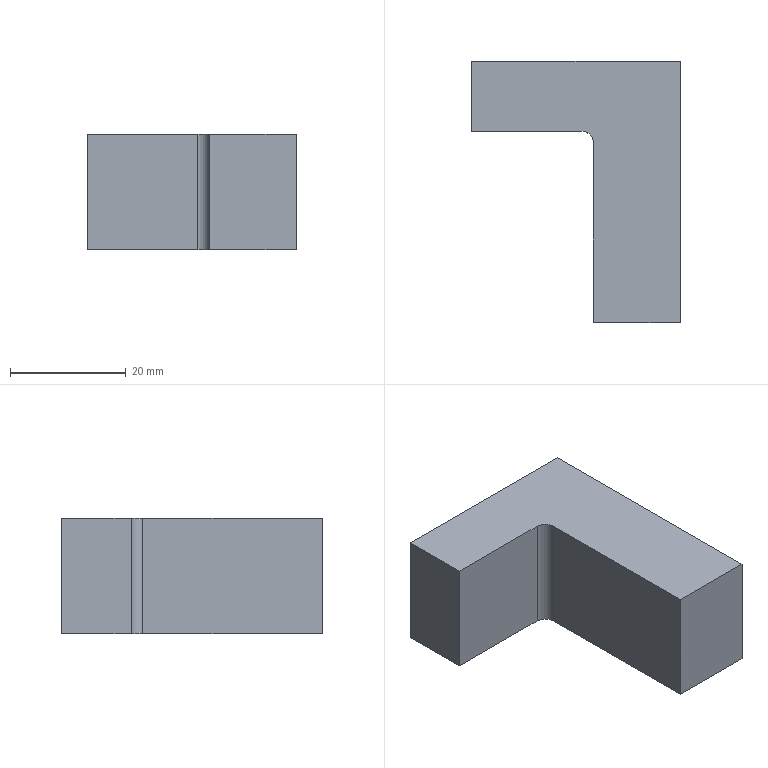Part | STEP file | 001-003-Shaft storage cylinder connection block | 1 solid | 9 faces | box 36 x 45 x 20 mm | volume 18557 mm3 | plane 8 | cylinder 1 | commonest cylinder face diameters 4 x1
STEP:
#1=CARTESIAN_POINT('',(0.,0.,0.));
#2=DIRECTION('',(0.,0.,1.));
#3=DIRECTION('',(1.,0.,0.));
#4=AXIS2_PLACEMENT_3D('',#1,#2,#3);
#5=CARTESIAN_POINT('',(18.,-22.5,0.));
#6=VERTEX_POINT('',#5);
#7=CARTESIAN_POINT('',(18.,22.5,0.));
#8=VERTEX_POINT('',#7);
#9=CARTESIAN_POINT('',(18.,-22.5,0.));
#10=DIRECTION('',(0.,1.,0.));
#11=VECTOR('',#10,1.);
#12=LINE('',#9,#11);
#13=CARTESIAN_POINT('',(18.,-22.5,20.));
#14=DIRECTION('',(-1.,0.,0.));
#15=DIRECTION('',(0.,0.,1.));
#16=AXIS2_PLACEMENT_3D('',#13,#14,#15);
#17=PLANE('',#16);
#18=CARTESIAN_POINT('',(-20.,0.));
#19=DIRECTION('',(0.,1.));
#20=VECTOR('',#19,1.);
#21=LINE('',#18,#20);
#22=(GEOMETRIC_REPRESENTATION_CONTEXT(2)PARAMETRIC_REPRESENTATION_CONTEXT()REPRESENTATION_CONTEXT('',''));
#23=DEFINITIONAL_REPRESENTATION('',(#21),#22);
#24=PCURVE('',#17,#23);
#25=CARTESIAN_POINT('',(0.,0.,0.));
#26=DIRECTION('',(0.,0.,-1.));
#27=DIRECTION('',(-1.,0.,0.));
#28=AXIS2_PLACEMENT_3D('',#25,#26,#27);
#29=PLANE('',#28);
#30=CARTESIAN_POINT('',(-18.,-22.5));
#31=DIRECTION('',(0.,1.));
#32=VECTOR('',#31,1.);
#33=LINE('',#30,#32);
#34=(GEOMETRIC_REPRESENTATION_CONTEXT(2)PARAMETRIC_REPRESENTATION_CONTEXT()REPRESENTATION_CONTEXT('',''));
#35=DEFINITIONAL_REPRESENTATION('',(#33),#34);
#36=PCURVE('',#29,#35);
#37=SURFACE_CURVE('',#12,(#24,#36),.PCURVE_S1.);
#38=EDGE_CURVE('',#6,#8,#37,.T.);
#39=ORIENTED_EDGE('',*,*,#38,.T.);
#40=CARTESIAN_POINT('',(18.,22.5,20.));
#41=VERTEX_POINT('',#40);
#42=CARTESIAN_POINT('',(18.,22.5,20.));
#43=DIRECTION('',(0.,0.,-1.));
#44=VECTOR('',#43,1.);
#45=LINE('',#42,#44);
#46=CARTESIAN_POINT('',(0.,45.));
#47=DIRECTION('',(-1.,0.));
#48=VECTOR('',#47,1.);
#49=LINE('',#46,#48);
#50=(GEOMETRIC_REPRESENTATION_CONTEXT(2)PARAMETRIC_REPRESENTATION_CONTEXT()REPRESENTATION_CONTEXT('',''));
#51=DEFINITIONAL_REPRESENTATION('',(#49),#50);
#52=PCURVE('',#17,#51);
#53=CARTESIAN_POINT('',(-18.,22.5,20.));
#54=DIRECTION('',(0.,-1.,0.));
#55=DIRECTION('',(0.,0.,-1.));
#56=AXIS2_PLACEMENT_3D('',#53,#54,#55);
#57=PLANE('',#56);
#58=CARTESIAN_POINT('',(0.,36.));
#59=DIRECTION('',(1.,0.));
#60=VECTOR('',#59,1.);
#61=LINE('',#58,#60);
#62=(GEOMETRIC_REPRESENTATION_CONTEXT(2)PARAMETRIC_REPRESENTATION_CONTEXT()REPRESENTATION_CONTEXT('',''));
#63=DEFINITIONAL_REPRESENTATION('',(#61),#62);
#64=PCURVE('',#57,#63);
#65=SURFACE_CURVE('',#45,(#52,#64),.PCURVE_S1.);
#66=EDGE_CURVE('',#41,#8,#65,.T.);
#67=ORIENTED_EDGE('',*,*,#66,.F.);
#68=CARTESIAN_POINT('',(18.,-22.5,20.));
#69=VERTEX_POINT('',#68);
#70=CARTESIAN_POINT('',(18.,-22.5,20.));
#71=DIRECTION('',(0.,1.,0.));
#72=VECTOR('',#71,1.);
#73=LINE('',#70,#72);
#74=CARTESIAN_POINT('',(0.,0.));
#75=DIRECTION('',(0.,1.));
#76=VECTOR('',#75,1.);
#77=LINE('',#74,#76);
#78=(GEOMETRIC_REPRESENTATION_CONTEXT(2)PARAMETRIC_REPRESENTATION_CONTEXT()REPRESENTATION_CONTEXT('',''));
#79=DEFINITIONAL_REPRESENTATION('',(#77),#78);
#80=PCURVE('',#17,#79);
#81=CARTESIAN_POINT('',(0.,0.,20.));
#82=DIRECTION('',(0.,0.,-1.));
#83=DIRECTION('',(-1.,0.,0.));
#84=AXIS2_PLACEMENT_3D('',#81,#82,#83);
#85=PLANE('',#84);
#86=CARTESIAN_POINT('',(-18.,-22.5));
#87=DIRECTION('',(0.,1.));
#88=VECTOR('',#87,1.);
#89=LINE('',#86,#88);
#90=(GEOMETRIC_REPRESENTATION_CONTEXT(2)PARAMETRIC_REPRESENTATION_CONTEXT()REPRESENTATION_CONTEXT('',''));
#91=DEFINITIONAL_REPRESENTATION('',(#89),#90);
#92=PCURVE('',#85,#91);
#93=SURFACE_CURVE('',#73,(#80,#92),.PCURVE_S1.);
#94=EDGE_CURVE('',#69,#41,#93,.T.);
#95=ORIENTED_EDGE('',*,*,#94,.F.);
#96=CARTESIAN_POINT('',(18.,-22.5,20.));
#97=DIRECTION('',(0.,0.,-1.));
#98=VECTOR('',#97,1.);
#99=LINE('',#96,#98);
#100=CARTESIAN_POINT('',(0.,0.));
#101=DIRECTION('',(-1.,0.));
#102=VECTOR('',#101,1.);
#103=LINE('',#100,#102);
#104=(GEOMETRIC_REPRESENTATION_CONTEXT(2)PARAMETRIC_REPRESENTATION_CONTEXT()REPRESENTATION_CONTEXT('',''));
#105=DEFINITIONAL_REPRESENTATION('',(#103),#104);
#106=PCURVE('',#17,#105);
#107=CARTESIAN_POINT('',(-18.,-22.5,20.));
#108=DIRECTION('',(0.,1.,0.));
#109=DIRECTION('',(0.,0.,1.));
#110=AXIS2_PLACEMENT_3D('',#107,#108,#109);
#111=PLANE('',#110);
#112=CARTESIAN_POINT('',(0.,36.));
#113=DIRECTION('',(-1.,0.));
#114=VECTOR('',#113,1.);
#115=LINE('',#112,#114);
#116=(GEOMETRIC_REPRESENTATION_CONTEXT(2)PARAMETRIC_REPRESENTATION_CONTEXT()REPRESENTATION_CONTEXT('',''));
#117=DEFINITIONAL_REPRESENTATION('',(#115),#116);
#118=PCURVE('',#111,#117);
#119=SURFACE_CURVE('',#99,(#106,#118),.PCURVE_S1.);
#120=EDGE_CURVE('',#69,#6,#119,.T.);
#121=ORIENTED_EDGE('',*,*,#120,.T.);
#122=EDGE_LOOP('',(#39,#67,#95,#121));
#123=FACE_BOUND('',#122,.T.);
#124=ADVANCED_FACE('',(#123),#17,.F.);
#125=CARTESIAN_POINT('',(-18.,22.5,0.));
#126=VERTEX_POINT('',#125);
#127=CARTESIAN_POINT('',(-18.,22.5,0.));
#128=DIRECTION('',(-1.,0.,0.));
#129=VECTOR('',#128,1.);
#130=LINE('',#127,#129);
#131=CARTESIAN_POINT('',(20.,0.));
#132=DIRECTION('',(0.,-1.));
#133=VECTOR('',#132,1.);
#134=LINE('',#131,#133);
#135=(GEOMETRIC_REPRESENTATION_CONTEXT(2)PARAMETRIC_REPRESENTATION_CONTEXT()REPRESENTATION_CONTEXT('',''));
#136=DEFINITIONAL_REPRESENTATION('',(#134),#135);
#137=PCURVE('',#57,#136);
#138=CARTESIAN_POINT('',(18.,22.5));
#139=DIRECTION('',(1.,0.));
#140=VECTOR('',#139,1.);
#141=LINE('',#138,#140);
#142=(GEOMETRIC_REPRESENTATION_CONTEXT(2)PARAMETRIC_REPRESENTATION_CONTEXT()REPRESENTATION_CONTEXT('',''));
#143=DEFINITIONAL_REPRESENTATION('',(#141),#142);
#144=PCURVE('',#29,#143);
#145=SURFACE_CURVE('',#130,(#137,#144),.PCURVE_S1.);
#146=EDGE_CURVE('',#8,#126,#145,.T.);
#147=ORIENTED_EDGE('',*,*,#146,.T.);
#148=CARTESIAN_POINT('',(-18.,22.5,20.));
#149=VERTEX_POINT('',#148);
#150=CARTESIAN_POINT('',(-18.,22.5,20.));
#151=DIRECTION('',(0.,0.,-1.));
#152=VECTOR('',#151,1.);
#153=LINE('',#150,#152);
#154=CARTESIAN_POINT('',(0.,0.));
#155=DIRECTION('',(1.,0.));
#156=VECTOR('',#155,1.);
#157=LINE('',#154,#156);
#158=(GEOMETRIC_REPRESENTATION_CONTEXT(2)PARAMETRIC_REPRESENTATION_CONTEXT()REPRESENTATION_CONTEXT('',''));
#159=DEFINITIONAL_REPRESENTATION('',(#157),#158);
#160=PCURVE('',#57,#159);
#161=CARTESIAN_POINT('',(-18.,-22.5,20.));
#162=DIRECTION('',(1.,0.,0.));
#163=DIRECTION('',(0.,0.,-1.));
#164=AXIS2_PLACEMENT_3D('',#161,#162,#163);
#165=PLANE('',#164);
#166=CARTESIAN_POINT('',(0.,45.));
#167=DIRECTION('',(1.,0.));
#168=VECTOR('',#167,1.);
#169=LINE('',#166,#168);
#170=(GEOMETRIC_REPRESENTATION_CONTEXT(2)PARAMETRIC_REPRESENTATION_CONTEXT()REPRESENTATION_CONTEXT('',''));
#171=DEFINITIONAL_REPRESENTATION('',(#169),#170);
#172=PCURVE('',#165,#171);
#173=SURFACE_CURVE('',#153,(#160,#172),.PCURVE_S1.);
#174=EDGE_CURVE('',#149,#126,#173,.T.);
#175=ORIENTED_EDGE('',*,*,#174,.F.);
#176=CARTESIAN_POINT('',(-18.,22.5,20.));
#177=DIRECTION('',(-1.,0.,0.));
#178=VECTOR('',#177,1.);
#179=LINE('',#176,#178);
#180=CARTESIAN_POINT('',(0.,0.));
#181=DIRECTION('',(0.,-1.));
#182=VECTOR('',#181,1.);
#183=LINE('',#180,#182);
#184=(GEOMETRIC_REPRESENTATION_CONTEXT(2)PARAMETRIC_REPRESENTATION_CONTEXT()REPRESENTATION_CONTEXT('',''));
#185=DEFINITIONAL_REPRESENTATION('',(#183),#184);
#186=PCURVE('',#57,#185);
#187=CARTESIAN_POINT('',(18.,22.5));
#188=DIRECTION('',(1.,0.));
#189=VECTOR('',#188,1.);
#190=LINE('',#187,#189);
#191=(GEOMETRIC_REPRESENTATION_CONTEXT(2)PARAMETRIC_REPRESENTATION_CONTEXT()REPRESENTATION_CONTEXT('',''));
#192=DEFINITIONAL_REPRESENTATION('',(#190),#191);
#193=PCURVE('',#85,#192);
#194=SURFACE_CURVE('',#179,(#186,#193),.PCURVE_S1.);
#195=EDGE_CURVE('',#41,#149,#194,.T.);
#196=ORIENTED_EDGE('',*,*,#195,.F.);
#197=ORIENTED_EDGE('',*,*,#66,.T.);
#198=EDGE_LOOP('',(#147,#175,#196,#197));
#199=FACE_BOUND('',#198,.T.);
#200=ADVANCED_FACE('',(#199),#57,.F.);
#201=CARTESIAN_POINT('',(-18.,10.5,0.));
#202=VERTEX_POINT('',#201);
#203=CARTESIAN_POINT('',(-18.,-22.5,0.));
#204=DIRECTION('',(0.,-1.,0.));
#205=VECTOR('',#204,1.);
#206=LINE('',#203,#205);
#207=CARTESIAN_POINT('',(20.,0.));
#208=DIRECTION('',(0.,-1.));
#209=VECTOR('',#208,1.);
#210=LINE('',#207,#209);
#211=(GEOMETRIC_REPRESENTATION_CONTEXT(2)PARAMETRIC_REPRESENTATION_CONTEXT()REPRESENTATION_CONTEXT('',''));
#212=DEFINITIONAL_REPRESENTATION('',(#210),#211);
#213=PCURVE('',#165,#212);
#214=CARTESIAN_POINT('',(18.,-22.5));
#215=DIRECTION('',(0.,-1.));
#216=VECTOR('',#215,1.);
#217=LINE('',#214,#216);
#218=(GEOMETRIC_REPRESENTATION_CONTEXT(2)PARAMETRIC_REPRESENTATION_CONTEXT()REPRESENTATION_CONTEXT('',''));
#219=DEFINITIONAL_REPRESENTATION('',(#217),#218);
#220=PCURVE('',#29,#219);
#221=SURFACE_CURVE('',#206,(#213,#220),.PCURVE_S1.);
#222=EDGE_CURVE('',#126,#202,#221,.T.);
#223=ORIENTED_EDGE('',*,*,#222,.T.);
#224=CARTESIAN_POINT('',(-18.,10.5,20.));
#225=VERTEX_POINT('',#224);
#226=CARTESIAN_POINT('',(-18.,10.5,0.));
#227=DIRECTION('',(0.,0.,1.));
#228=VECTOR('',#227,1.);
#229=LINE('',#226,#228);
#230=CARTESIAN_POINT('',(20.,33.));
#231=DIRECTION('',(-1.,0.));
#232=VECTOR('',#231,1.);
#233=LINE('',#230,#232);
#234=(GEOMETRIC_REPRESENTATION_CONTEXT(2)PARAMETRIC_REPRESENTATION_CONTEXT()REPRESENTATION_CONTEXT('',''));
#235=DEFINITIONAL_REPRESENTATION('',(#233),#234);
#236=PCURVE('',#165,#235);
#237=CARTESIAN_POINT('',(-18.,10.5,0.));
#238=DIRECTION('',(0.,1.,0.));
#239=DIRECTION('',(0.,0.,1.));
#240=AXIS2_PLACEMENT_3D('',#237,#238,#239);
#241=PLANE('',#240);
#242=CARTESIAN_POINT('',(0.,0.));
#243=DIRECTION('',(1.,0.));
#244=VECTOR('',#243,1.);
#245=LINE('',#242,#244);
#246=(GEOMETRIC_REPRESENTATION_CONTEXT(2)PARAMETRIC_REPRESENTATION_CONTEXT()REPRESENTATION_CONTEXT('',''));
#247=DEFINITIONAL_REPRESENTATION('',(#245),#246);
#248=PCURVE('',#241,#247);
#249=SURFACE_CURVE('',#229,(#236,#248),.PCURVE_S1.);
#250=EDGE_CURVE('',#202,#225,#249,.T.);
#251=ORIENTED_EDGE('',*,*,#250,.T.);
#252=CARTESIAN_POINT('',(-18.,-22.5,20.));
#253=DIRECTION('',(0.,-1.,0.));
#254=VECTOR('',#253,1.);
#255=LINE('',#252,#254);
#256=CARTESIAN_POINT('',(0.,0.));
#257=DIRECTION('',(0.,-1.));
#258=VECTOR('',#257,1.);
#259=LINE('',#256,#258);
#260=(GEOMETRIC_REPRESENTATION_CONTEXT(2)PARAMETRIC_REPRESENTATION_CONTEXT()REPRESENTATION_CONTEXT('',''));
#261=DEFINITIONAL_REPRESENTATION('',(#259),#260);
#262=PCURVE('',#165,#261);
#263=CARTESIAN_POINT('',(18.,-22.5));
#264=DIRECTION('',(0.,-1.));
#265=VECTOR('',#264,1.);
#266=LINE('',#263,#265);
#267=(GEOMETRIC_REPRESENTATION_CONTEXT(2)PARAMETRIC_REPRESENTATION_CONTEXT()REPRESENTATION_CONTEXT('',''));
#268=DEFINITIONAL_REPRESENTATION('',(#266),#267);
#269=PCURVE('',#85,#268);
#270=SURFACE_CURVE('',#255,(#262,#269),.PCURVE_S1.);
#271=EDGE_CURVE('',#149,#225,#270,.T.);
#272=ORIENTED_EDGE('',*,*,#271,.F.);
#273=ORIENTED_EDGE('',*,*,#174,.T.);
#274=EDGE_LOOP('',(#223,#251,#272,#273));
#275=FACE_BOUND('',#274,.T.);
#276=ADVANCED_FACE('',(#275),#165,.F.);
#277=CARTESIAN_POINT('',(3.,-22.5,20.));
#278=VERTEX_POINT('',#277);
#279=CARTESIAN_POINT('',(-18.,-22.5,20.));
#280=DIRECTION('',(1.,0.,0.));
#281=VECTOR('',#280,1.);
#282=LINE('',#279,#281);
#283=CARTESIAN_POINT('',(0.,0.));
#284=DIRECTION('',(0.,1.));
#285=VECTOR('',#284,1.);
#286=LINE('',#283,#285);
#287=(GEOMETRIC_REPRESENTATION_CONTEXT(2)PARAMETRIC_REPRESENTATION_CONTEXT()REPRESENTATION_CONTEXT('',''));
#288=DEFINITIONAL_REPRESENTATION('',(#286),#287);
#289=PCURVE('',#111,#288);
#290=CARTESIAN_POINT('',(18.,-22.5));
#291=DIRECTION('',(-1.,0.));
#292=VECTOR('',#291,1.);
#293=LINE('',#290,#292);
#294=(GEOMETRIC_REPRESENTATION_CONTEXT(2)PARAMETRIC_REPRESENTATION_CONTEXT()REPRESENTATION_CONTEXT('',''));
#295=DEFINITIONAL_REPRESENTATION('',(#293),#294);
#296=PCURVE('',#85,#295);
#297=SURFACE_CURVE('',#282,(#289,#296),.PCURVE_S1.);
#298=EDGE_CURVE('',#278,#69,#297,.T.);
#299=ORIENTED_EDGE('',*,*,#298,.F.);
#300=CARTESIAN_POINT('',(3.,-22.5,0.));
#301=VERTEX_POINT('',#300);
#302=CARTESIAN_POINT('',(3.,-22.5,0.));
#303=DIRECTION('',(0.,0.,1.));
#304=VECTOR('',#303,1.);
#305=LINE('',#302,#304);
#306=CARTESIAN_POINT('',(-20.,21.));
#307=DIRECTION('',(1.,0.));
#308=VECTOR('',#307,1.);
#309=LINE('',#306,#308);
#310=(GEOMETRIC_REPRESENTATION_CONTEXT(2)PARAMETRIC_REPRESENTATION_CONTEXT()REPRESENTATION_CONTEXT('',''));
#311=DEFINITIONAL_REPRESENTATION('',(#309),#310);
#312=PCURVE('',#111,#311);
#313=CARTESIAN_POINT('',(3.,-22.5,0.));
#314=DIRECTION('',(1.,0.,0.));
#315=DIRECTION('',(0.,0.,-1.));
#316=AXIS2_PLACEMENT_3D('',#313,#314,#315);
#317=PLANE('',#316);
#318=CARTESIAN_POINT('',(0.,0.));
#319=DIRECTION('',(-1.,0.));
#320=VECTOR('',#319,1.);
#321=LINE('',#318,#320);
#322=(GEOMETRIC_REPRESENTATION_CONTEXT(2)PARAMETRIC_REPRESENTATION_CONTEXT()REPRESENTATION_CONTEXT('',''));
#323=DEFINITIONAL_REPRESENTATION('',(#321),#322);
#324=PCURVE('',#317,#323);
#325=SURFACE_CURVE('',#305,(#312,#324),.PCURVE_S1.);
#326=EDGE_CURVE('',#301,#278,#325,.T.);
#327=ORIENTED_EDGE('',*,*,#326,.F.);
#328=CARTESIAN_POINT('',(-18.,-22.5,0.));
#329=DIRECTION('',(1.,0.,0.));
#330=VECTOR('',#329,1.);
#331=LINE('',#328,#330);
#332=CARTESIAN_POINT('',(-20.,0.));
#333=DIRECTION('',(0.,1.));
#334=VECTOR('',#333,1.);
#335=LINE('',#332,#334);
#336=(GEOMETRIC_REPRESENTATION_CONTEXT(2)PARAMETRIC_REPRESENTATION_CONTEXT()REPRESENTATION_CONTEXT('',''));
#337=DEFINITIONAL_REPRESENTATION('',(#335),#336);
#338=PCURVE('',#111,#337);
#339=CARTESIAN_POINT('',(18.,-22.5));
#340=DIRECTION('',(-1.,0.));
#341=VECTOR('',#340,1.);
#342=LINE('',#339,#341);
#343=(GEOMETRIC_REPRESENTATION_CONTEXT(2)PARAMETRIC_REPRESENTATION_CONTEXT()REPRESENTATION_CONTEXT('',''));
#344=DEFINITIONAL_REPRESENTATION('',(#342),#343);
#345=PCURVE('',#29,#344);
#346=SURFACE_CURVE('',#331,(#338,#345),.PCURVE_S1.);
#347=EDGE_CURVE('',#301,#6,#346,.T.);
#348=ORIENTED_EDGE('',*,*,#347,.T.);
#349=ORIENTED_EDGE('',*,*,#120,.F.);
#350=EDGE_LOOP('',(#299,#327,#348,#349));
#351=FACE_BOUND('',#350,.T.);
#352=ADVANCED_FACE('',(#351),#111,.F.);
#353=ORIENTED_EDGE('',*,*,#271,.T.);
#354=CARTESIAN_POINT('',(1.,10.5,20.));
#355=VERTEX_POINT('',#354);
#356=CARTESIAN_POINT('',(-18.,10.5,20.));
#357=DIRECTION('',(-1.,0.,0.));
#358=VECTOR('',#357,1.);
#359=LINE('',#356,#358);
#360=CARTESIAN_POINT('',(18.,10.5));
#361=DIRECTION('',(1.,0.));
#362=VECTOR('',#361,1.);
#363=LINE('',#360,#362);
#364=(GEOMETRIC_REPRESENTATION_CONTEXT(2)PARAMETRIC_REPRESENTATION_CONTEXT()REPRESENTATION_CONTEXT('',''));
#365=DEFINITIONAL_REPRESENTATION('',(#363),#364);
#366=PCURVE('',#85,#365);
#367=CARTESIAN_POINT('',(20.,0.));
#368=DIRECTION('',(0.,-1.));
#369=VECTOR('',#368,1.);
#370=LINE('',#367,#369);
#371=(GEOMETRIC_REPRESENTATION_CONTEXT(2)PARAMETRIC_REPRESENTATION_CONTEXT()REPRESENTATION_CONTEXT('',''));
#372=DEFINITIONAL_REPRESENTATION('',(#370),#371);
#373=PCURVE('',#241,#372);
#374=SURFACE_CURVE('',#359,(#366,#373),.PCURVE_S1.);
#375=EDGE_CURVE('',#355,#225,#374,.T.);
#376=ORIENTED_EDGE('',*,*,#375,.F.);
#377=CARTESIAN_POINT('',(3.,8.5,20.));
#378=VERTEX_POINT('',#377);
#379=CARTESIAN_POINT('',(1.,8.5,20.));
#380=DIRECTION('',(0.,0.,-1.));
#381=DIRECTION('',(-1.,0.,0.));
#382=AXIS2_PLACEMENT_3D('',#379,#380,#381);
#383=CIRCLE('',#382,2.);
#384=CARTESIAN_POINT('',(-1.,8.5));
#385=DIRECTION('',(1.,0.));
#386=AXIS2_PLACEMENT_2D('',#384,#385);
#387=CIRCLE('',#386,2.);
#388=(GEOMETRIC_REPRESENTATION_CONTEXT(2)PARAMETRIC_REPRESENTATION_CONTEXT()REPRESENTATION_CONTEXT('',''));
#389=DEFINITIONAL_REPRESENTATION('',(#387),#388);
#390=PCURVE('',#85,#389);
#391=CARTESIAN_POINT('',(1.,8.5,0.));
#392=DIRECTION('',(0.,0.,-1.));
#393=DIRECTION('',(-1.,0.,0.));
#394=AXIS2_PLACEMENT_3D('',#391,#392,#393);
#395=CYLINDRICAL_SURFACE('',#394,2.);
#396=CARTESIAN_POINT('',(0.,-20.));
#397=DIRECTION('',(1.,0.));
#398=VECTOR('',#397,1.);
#399=LINE('',#396,#398);
#400=(GEOMETRIC_REPRESENTATION_CONTEXT(2)PARAMETRIC_REPRESENTATION_CONTEXT()REPRESENTATION_CONTEXT('',''));
#401=DEFINITIONAL_REPRESENTATION('',(#399),#400);
#402=PCURVE('',#395,#401);
#403=SURFACE_CURVE('',#383,(#390,#402),.PCURVE_S1.);
#404=EDGE_CURVE('',#355,#378,#403,.T.);
#405=ORIENTED_EDGE('',*,*,#404,.T.);
#406=CARTESIAN_POINT('',(3.,-22.5,20.));
#407=DIRECTION('',(0.,1.,0.));
#408=VECTOR('',#407,1.);
#409=LINE('',#406,#408);
#410=CARTESIAN_POINT('',(-3.,-22.5));
#411=DIRECTION('',(0.,1.));
#412=VECTOR('',#411,1.);
#413=LINE('',#410,#412);
#414=(GEOMETRIC_REPRESENTATION_CONTEXT(2)PARAMETRIC_REPRESENTATION_CONTEXT()REPRESENTATION_CONTEXT('',''));
#415=DEFINITIONAL_REPRESENTATION('',(#413),#414);
#416=PCURVE('',#85,#415);
#417=CARTESIAN_POINT('',(-20.,0.));
#418=DIRECTION('',(0.,1.));
#419=VECTOR('',#418,1.);
#420=LINE('',#417,#419);
#421=(GEOMETRIC_REPRESENTATION_CONTEXT(2)PARAMETRIC_REPRESENTATION_CONTEXT()REPRESENTATION_CONTEXT('',''));
#422=DEFINITIONAL_REPRESENTATION('',(#420),#421);
#423=PCURVE('',#317,#422);
#424=SURFACE_CURVE('',#409,(#416,#423),.PCURVE_S1.);
#425=EDGE_CURVE('',#278,#378,#424,.T.);
#426=ORIENTED_EDGE('',*,*,#425,.F.);
#427=ORIENTED_EDGE('',*,*,#298,.T.);
#428=ORIENTED_EDGE('',*,*,#94,.T.);
#429=ORIENTED_EDGE('',*,*,#195,.T.);
#430=EDGE_LOOP('',(#353,#376,#405,#426,#427,#428,#429));
#431=FACE_BOUND('',#430,.T.);
#432=ADVANCED_FACE('',(#431),#85,.F.);
#433=CARTESIAN_POINT('',(3.,8.5,0.));
#434=VERTEX_POINT('',#433);
#435=CARTESIAN_POINT('',(3.,-22.5,0.));
#436=DIRECTION('',(0.,1.,0.));
#437=VECTOR('',#436,1.);
#438=LINE('',#435,#437);
#439=CARTESIAN_POINT('',(-3.,-22.5));
#440=DIRECTION('',(0.,1.));
#441=VECTOR('',#440,1.);
#442=LINE('',#439,#441);
#443=(GEOMETRIC_REPRESENTATION_CONTEXT(2)PARAMETRIC_REPRESENTATION_CONTEXT()REPRESENTATION_CONTEXT('',''));
#444=DEFINITIONAL_REPRESENTATION('',(#442),#443);
#445=PCURVE('',#29,#444);
#446=CARTESIAN_POINT('',(0.,0.));
#447=DIRECTION('',(0.,1.));
#448=VECTOR('',#447,1.);
#449=LINE('',#446,#448);
#450=(GEOMETRIC_REPRESENTATION_CONTEXT(2)PARAMETRIC_REPRESENTATION_CONTEXT()REPRESENTATION_CONTEXT('',''));
#451=DEFINITIONAL_REPRESENTATION('',(#449),#450);
#452=PCURVE('',#317,#451);
#453=SURFACE_CURVE('',#438,(#445,#452),.PCURVE_S1.);
#454=EDGE_CURVE('',#301,#434,#453,.T.);
#455=ORIENTED_EDGE('',*,*,#454,.T.);
#456=CARTESIAN_POINT('',(1.,10.5,0.));
#457=VERTEX_POINT('',#456);
#458=CARTESIAN_POINT('',(1.,8.5,0.));
#459=DIRECTION('',(0.,0.,1.));
#460=DIRECTION('',(-1.,0.,0.));
#461=AXIS2_PLACEMENT_3D('',#458,#459,#460);
#462=CIRCLE('',#461,2.);
#463=CARTESIAN_POINT('',(1.,8.5));
#464=CARTESIAN_POINT('',(1.,5.036));
#465=CARTESIAN_POINT('',(-2.,6.768));
#466=CARTESIAN_POINT('',(-5.,8.5));
#467=CARTESIAN_POINT('',(-2.,10.232));
#468=CARTESIAN_POINT('',(1.,11.964));
#469=CARTESIAN_POINT('',(1.,8.5));
#470=(BOUNDED_CURVE()B_SPLINE_CURVE(2,(#463,#464,#465,#466,#467,#468,#469),.UNSPECIFIED.,.T.,.F.)B_SPLINE_CURVE_WITH_KNOTS((1,2,2,2,2,1),(-2.094,0.,2.094,4.189,6.283,8.378),.UNSPECIFIED.)CURVE()GEOMETRIC_REPRESENTATION_ITEM()RATIONAL_B_SPLINE_CURVE((1.,0.5,1.,0.5,1.,0.5,1.))REPRESENTATION_ITEM(''));
#471=(GEOMETRIC_REPRESENTATION_CONTEXT(2)PARAMETRIC_REPRESENTATION_CONTEXT()REPRESENTATION_CONTEXT('',''));
#472=DEFINITIONAL_REPRESENTATION('',(#470),#471);
#473=PCURVE('',#29,#472);
#474=CARTESIAN_POINT('',(6.283,0.));
#475=DIRECTION('',(-1.,0.));
#476=VECTOR('',#475,1.);
#477=LINE('',#474,#476);
#478=(GEOMETRIC_REPRESENTATION_CONTEXT(2)PARAMETRIC_REPRESENTATION_CONTEXT()REPRESENTATION_CONTEXT('',''));
#479=DEFINITIONAL_REPRESENTATION('',(#477),#478);
#480=PCURVE('',#395,#479);
#481=SURFACE_CURVE('',#462,(#473,#480),.PCURVE_S1.);
#482=EDGE_CURVE('',#434,#457,#481,.T.);
#483=ORIENTED_EDGE('',*,*,#482,.T.);
#484=CARTESIAN_POINT('',(-18.,10.5,0.));
#485=DIRECTION('',(-1.,0.,0.));
#486=VECTOR('',#485,1.);
#487=LINE('',#484,#486);
#488=CARTESIAN_POINT('',(18.,10.5));
#489=DIRECTION('',(1.,0.));
#490=VECTOR('',#489,1.);
#491=LINE('',#488,#490);
#492=(GEOMETRIC_REPRESENTATION_CONTEXT(2)PARAMETRIC_REPRESENTATION_CONTEXT()REPRESENTATION_CONTEXT('',''));
#493=DEFINITIONAL_REPRESENTATION('',(#491),#492);
#494=PCURVE('',#29,#493);
#495=CARTESIAN_POINT('',(0.,0.));
#496=DIRECTION('',(0.,-1.));
#497=VECTOR('',#496,1.);
#498=LINE('',#495,#497);
#499=(GEOMETRIC_REPRESENTATION_CONTEXT(2)PARAMETRIC_REPRESENTATION_CONTEXT()REPRESENTATION_CONTEXT('',''));
#500=DEFINITIONAL_REPRESENTATION('',(#498),#499);
#501=PCURVE('',#241,#500);
#502=SURFACE_CURVE('',#487,(#494,#501),.PCURVE_S1.);
#503=EDGE_CURVE('',#457,#202,#502,.T.);
#504=ORIENTED_EDGE('',*,*,#503,.T.);
#505=ORIENTED_EDGE('',*,*,#222,.F.);
#506=ORIENTED_EDGE('',*,*,#146,.F.);
#507=ORIENTED_EDGE('',*,*,#38,.F.);
#508=ORIENTED_EDGE('',*,*,#347,.F.);
#509=EDGE_LOOP('',(#455,#483,#504,#505,#506,#507,#508));
#510=FACE_BOUND('',#509,.T.);
#511=ADVANCED_FACE('',(#510),#29,.T.);
#512=ORIENTED_EDGE('',*,*,#503,.F.);
#513=CARTESIAN_POINT('',(1.,10.5,20.));
#514=DIRECTION('',(0.,0.,1.));
#515=VECTOR('',#514,1.);
#516=LINE('',#513,#515);
#517=CARTESIAN_POINT('',(20.,19.));
#518=DIRECTION('',(1.,0.));
#519=VECTOR('',#518,1.);
#520=LINE('',#517,#519);
#521=(GEOMETRIC_REPRESENTATION_CONTEXT(2)PARAMETRIC_REPRESENTATION_CONTEXT()REPRESENTATION_CONTEXT('',''));
#522=DEFINITIONAL_REPRESENTATION('',(#520),#521);
#523=PCURVE('',#241,#522);
#524=CARTESIAN_POINT('',(1.571,-20.));
#525=DIRECTION('',(0.,-1.));
#526=VECTOR('',#525,1.);
#527=LINE('',#524,#526);
#528=(GEOMETRIC_REPRESENTATION_CONTEXT(2)PARAMETRIC_REPRESENTATION_CONTEXT()REPRESENTATION_CONTEXT('',''));
#529=DEFINITIONAL_REPRESENTATION('',(#527),#528);
#530=PCURVE('',#395,#529);
#531=SURFACE_CURVE('',#516,(#523,#530),.PCURVE_S1.);
#532=EDGE_CURVE('',#457,#355,#531,.T.);
#533=ORIENTED_EDGE('',*,*,#532,.T.);
#534=ORIENTED_EDGE('',*,*,#375,.T.);
#535=ORIENTED_EDGE('',*,*,#250,.F.);
#536=EDGE_LOOP('',(#512,#533,#534,#535));
#537=FACE_BOUND('',#536,.T.);
#538=ADVANCED_FACE('',(#537),#241,.F.);
#539=ORIENTED_EDGE('',*,*,#425,.T.);
#540=CARTESIAN_POINT('',(3.,8.5,0.));
#541=DIRECTION('',(0.,0.,-1.));
#542=VECTOR('',#541,1.);
#543=LINE('',#540,#542);
#544=CARTESIAN_POINT('',(0.,31.));
#545=DIRECTION('',(1.,0.));
#546=VECTOR('',#545,1.);
#547=LINE('',#544,#546);
#548=(GEOMETRIC_REPRESENTATION_CONTEXT(2)PARAMETRIC_REPRESENTATION_CONTEXT()REPRESENTATION_CONTEXT('',''));
#549=DEFINITIONAL_REPRESENTATION('',(#547),#548);
#550=PCURVE('',#317,#549);
#551=CARTESIAN_POINT('',(3.142,0.));
#552=DIRECTION('',(0.,1.));
#553=VECTOR('',#552,1.);
#554=LINE('',#551,#553);
#555=(GEOMETRIC_REPRESENTATION_CONTEXT(2)PARAMETRIC_REPRESENTATION_CONTEXT()REPRESENTATION_CONTEXT('',''));
#556=DEFINITIONAL_REPRESENTATION('',(#554),#555);
#557=PCURVE('',#395,#556);
#558=SURFACE_CURVE('',#543,(#550,#557),.PCURVE_S1.);
#559=EDGE_CURVE('',#378,#434,#558,.T.);
#560=ORIENTED_EDGE('',*,*,#559,.T.);
#561=ORIENTED_EDGE('',*,*,#454,.F.);
#562=ORIENTED_EDGE('',*,*,#326,.T.);
#563=EDGE_LOOP('',(#539,#560,#561,#562));
#564=FACE_BOUND('',#563,.T.);
#565=ADVANCED_FACE('',(#564),#317,.F.);
#566=ORIENTED_EDGE('',*,*,#532,.T.);
#567=ORIENTED_EDGE('',*,*,#404,.T.);
#568=ORIENTED_EDGE('',*,*,#559,.T.);
#569=ORIENTED_EDGE('',*,*,#482,.T.);
#570=EDGE_LOOP('',(#566,#567,#568,#569));
#571=FACE_BOUND('',#570,.F.);
#572=ADVANCED_FACE('',(#571),#395,.F.);
#573=CLOSED_SHELL('',(#124,#200,#276,#352,#432,#511,#538,#565,#572));
#574=MANIFOLD_SOLID_BREP('',#573);
#575=(LENGTH_UNIT()NAMED_UNIT(*)SI_UNIT(.MILLI.,.METRE.));
#576=UNCERTAINTY_MEASURE_WITH_UNIT(LENGTH_MEASURE(0.0000001),#575,'','');
#577=(NAMED_UNIT(*)PLANE_ANGLE_UNIT()SI_UNIT($,.RADIAN.));
#578=(NAMED_UNIT(*)SI_UNIT($,.STERADIAN.)SOLID_ANGLE_UNIT());
#579=(GEOMETRIC_REPRESENTATION_CONTEXT(3)GLOBAL_UNCERTAINTY_ASSIGNED_CONTEXT((#576))GLOBAL_UNIT_ASSIGNED_CONTEXT((#575,#577,#578))REPRESENTATION_CONTEXT('',''));
#580=ADVANCED_BREP_SHAPE_REPRESENTATION('',(#4,#574),#579);